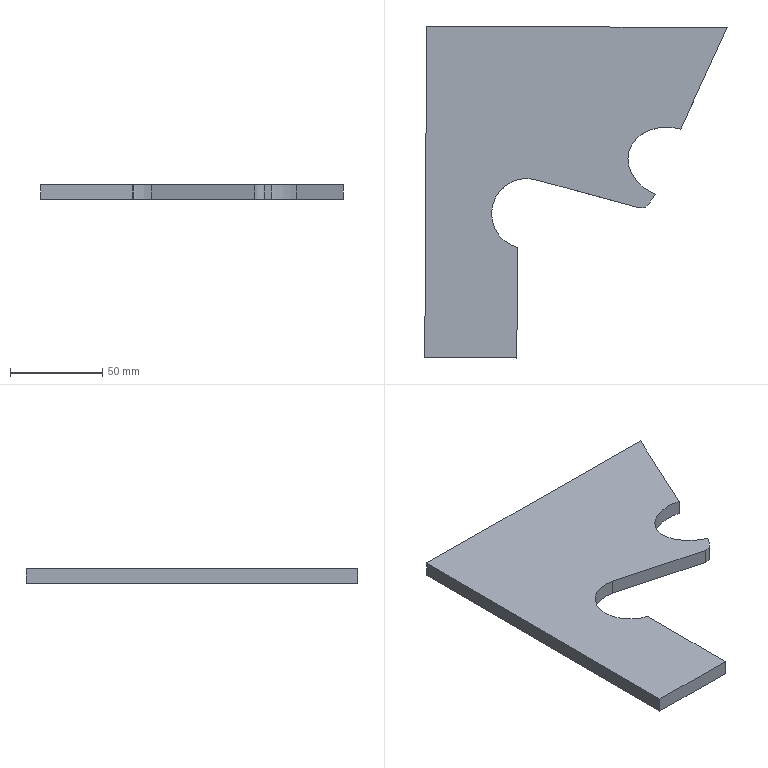Part | SolidWorks | features FlatPattern 1, SMBaseFlange 1, SheetMetal 1 | 1 solid | 14 faces | box 164.239 x 180.27 x 8 mm | volume 131142 mm3 | plane 9 | cylinder 3 | spline 2 | commonest cylinder face diameters 38.1 x2 10 x1
STEP:
#1=CARTESIAN_POINT('',(-214.283,4.192,8.));
#2=VERTEX_POINT('',#1);
#3=CARTESIAN_POINT('',(-190.247,22.578,8.));
#4=VERTEX_POINT('',#3);
#5=CARTESIAN_POINT('',(-195.233,4.192,8.));
#6=DIRECTION('',(0.,0.,-1.));
#7=DIRECTION('',(1.,0.,0.));
#8=AXIS2_PLACEMENT_3D('',#5,#6,#7);
#9=CIRCLE('',#8,19.05);
#10=EDGE_CURVE('',#2,#4,#9,.T.);
#11=ORIENTED_EDGE('',*,*,#10,.F.);
#12=CARTESIAN_POINT('',(-214.283,4.192,0.));
#13=VERTEX_POINT('',#12);
#14=CARTESIAN_POINT('',(-214.283,4.192,8.));
#15=DIRECTION('',(0.,0.,-1.));
#16=VECTOR('',#15,1000.);
#17=LINE('',#14,#16);
#18=EDGE_CURVE('',#2,#13,#17,.T.);
#19=ORIENTED_EDGE('',*,*,#18,.T.);
#20=CARTESIAN_POINT('',(-190.247,22.578,0.));
#21=VERTEX_POINT('',#20);
#22=CARTESIAN_POINT('',(-195.233,4.192,0.));
#23=DIRECTION('',(0.,0.,-1.));
#24=DIRECTION('',(1.,0.,0.));
#25=AXIS2_PLACEMENT_3D('',#22,#23,#24);
#26=CIRCLE('',#25,19.05);
#27=EDGE_CURVE('',#13,#21,#26,.T.);
#28=ORIENTED_EDGE('',*,*,#27,.T.);
#29=CARTESIAN_POINT('',(-190.247,22.578,8.));
#30=DIRECTION('',(0.,0.,-1.));
#31=VECTOR('',#30,1000.);
#32=LINE('',#29,#31);
#33=EDGE_CURVE('',#4,#21,#32,.T.);
#34=ORIENTED_EDGE('',*,*,#33,.F.);
#35=EDGE_LOOP('',(#11,#19,#28,#34));
#36=FACE_OUTER_BOUND('',#35,.T.);
#37=CARTESIAN_POINT('',(-195.233,4.192,8.));
#38=DIRECTION('',(0.,0.,-1.));
#39=DIRECTION('',(-1.,0.,0.));
#40=AXIS2_PLACEMENT_3D('',#37,#38,#39);
#41=CYLINDRICAL_SURFACE('',#40,19.05);
#42=ADVANCED_FACE('',(#36),#41,.F.);
#43=CARTESIAN_POINT('',(-139.675,37.946,8.));
#44=VERTEX_POINT('',#43);
#45=CARTESIAN_POINT('',(-111.658,50.087,8.));
#46=VERTEX_POINT('',#45);
#47=CARTESIAN_POINT('',(-139.675,37.946,8.));
#48=CARTESIAN_POINT('',(-136.754,48.717,8.));
#49=CARTESIAN_POINT('',(-125.15,53.746,8.));
#50=CARTESIAN_POINT('',(-111.658,50.087,8.));
#51=(BOUNDED_CURVE()B_SPLINE_CURVE(3,(#47,#48,#49,#50),.UNSPECIFIED.,.F.,.F.)B_SPLINE_CURVE_WITH_KNOTS((4,4),(0.,1.571),.UNSPECIFIED.)CURVE()GEOMETRIC_REPRESENTATION_ITEM()RATIONAL_B_SPLINE_CURVE((1.,0.8047,0.8047,1.))REPRESENTATION_ITEM(''));
#52=EDGE_CURVE('',#44,#46,#51,.T.);
#53=ORIENTED_EDGE('',*,*,#52,.F.);
#54=CARTESIAN_POINT('',(-139.675,37.946,0.));
#55=VERTEX_POINT('',#54);
#56=CARTESIAN_POINT('',(-139.675,37.946,8.));
#57=DIRECTION('',(0.,0.,-1.));
#58=VECTOR('',#57,1000.);
#59=LINE('',#56,#58);
#60=EDGE_CURVE('',#44,#55,#59,.T.);
#61=ORIENTED_EDGE('',*,*,#60,.T.);
#62=CARTESIAN_POINT('',(-111.658,50.087,0.));
#63=VERTEX_POINT('',#62);
#64=CARTESIAN_POINT('',(-139.675,37.946,0.));
#65=CARTESIAN_POINT('',(-136.754,48.717,0.));
#66=CARTESIAN_POINT('',(-125.15,53.746,0.));
#67=CARTESIAN_POINT('',(-111.658,50.087,0.));
#68=(BOUNDED_CURVE()B_SPLINE_CURVE(3,(#64,#65,#66,#67),.UNSPECIFIED.,.F.,.F.)B_SPLINE_CURVE_WITH_KNOTS((4,4),(0.,1.571),.UNSPECIFIED.)CURVE()GEOMETRIC_REPRESENTATION_ITEM()RATIONAL_B_SPLINE_CURVE((1.,0.8047,0.8047,1.))REPRESENTATION_ITEM(''));
#69=EDGE_CURVE('',#55,#63,#68,.T.);
#70=ORIENTED_EDGE('',*,*,#69,.T.);
#71=CARTESIAN_POINT('',(-111.658,50.087,8.));
#72=DIRECTION('',(0.,0.,-1.));
#73=VECTOR('',#72,1000.);
#74=LINE('',#71,#73);
#75=EDGE_CURVE('',#46,#63,#74,.T.);
#76=ORIENTED_EDGE('',*,*,#75,.F.);
#77=EDGE_LOOP('',(#53,#61,#70,#76));
#78=FACE_OUTER_BOUND('',#77,.T.);
#79=CARTESIAN_POINT('',(-139.675,37.946,8.));
#80=CARTESIAN_POINT('',(-139.675,37.946,0.));
#81=CARTESIAN_POINT('',(-136.754,48.717,8.));
#82=CARTESIAN_POINT('',(-136.754,48.717,0.));
#83=CARTESIAN_POINT('',(-125.15,53.746,8.));
#84=CARTESIAN_POINT('',(-125.15,53.746,0.));
#85=CARTESIAN_POINT('',(-111.658,50.087,8.));
#86=CARTESIAN_POINT('',(-111.658,50.087,0.));
#87=(BOUNDED_SURFACE()B_SPLINE_SURFACE(3,1,((#79,#80),(#81,#82),(#83,#84),(#85,#86)),.UNSPECIFIED.,.F.,.F.,.F.)B_SPLINE_SURFACE_WITH_KNOTS((4,4),(2,2),(0.,1.),(0.,1.),.UNSPECIFIED.)GEOMETRIC_REPRESENTATION_ITEM()RATIONAL_B_SPLINE_SURFACE(((1.,1.),(0.8047,0.8047),(0.8047,0.8047),(1.,1.)))REPRESENTATION_ITEM('')SURFACE());
#88=ADVANCED_FACE('',(#78),#87,.F.);
#89=ORIENTED_EDGE('',*,*,#60,.F.);
#90=CARTESIAN_POINT('',(-125.259,14.555,8.));
#91=VERTEX_POINT('',#90);
#92=CARTESIAN_POINT('',(-125.259,14.555,8.));
#93=CARTESIAN_POINT('',(-136.522,19.235,8.));
#94=CARTESIAN_POINT('',(-142.235,28.505,8.));
#95=CARTESIAN_POINT('',(-139.675,37.946,8.));
#96=(BOUNDED_CURVE()B_SPLINE_CURVE(3,(#92,#93,#94,#95),.UNSPECIFIED.,.F.,.F.)B_SPLINE_CURVE_WITH_KNOTS((4,4),(4.874,6.283),.UNSPECIFIED.)CURVE()GEOMETRIC_REPRESENTATION_ITEM()RATIONAL_B_SPLINE_CURVE((1.,0.8411,0.8411,1.))REPRESENTATION_ITEM(''));
#97=EDGE_CURVE('',#91,#44,#96,.T.);
#98=ORIENTED_EDGE('',*,*,#97,.F.);
#99=CARTESIAN_POINT('',(-125.259,14.555,0.));
#100=VERTEX_POINT('',#99);
#101=CARTESIAN_POINT('',(-125.259,14.555,8.));
#102=DIRECTION('',(0.,0.,-1.));
#103=VECTOR('',#102,1000.);
#104=LINE('',#101,#103);
#105=EDGE_CURVE('',#91,#100,#104,.T.);
#106=ORIENTED_EDGE('',*,*,#105,.T.);
#107=CARTESIAN_POINT('',(-125.259,14.555,0.));
#108=CARTESIAN_POINT('',(-136.522,19.235,0.));
#109=CARTESIAN_POINT('',(-142.235,28.505,0.));
#110=CARTESIAN_POINT('',(-139.675,37.946,0.));
#111=(BOUNDED_CURVE()B_SPLINE_CURVE(3,(#107,#108,#109,#110),.UNSPECIFIED.,.F.,.T.)B_SPLINE_CURVE_WITH_KNOTS((4,4),(4.874,6.283),.UNSPECIFIED.)CURVE()GEOMETRIC_REPRESENTATION_ITEM()RATIONAL_B_SPLINE_CURVE((1.,0.8411,0.8411,1.))REPRESENTATION_ITEM(''));
#112=EDGE_CURVE('',#100,#55,#111,.T.);
#113=ORIENTED_EDGE('',*,*,#112,.T.);
#114=EDGE_LOOP('',(#89,#98,#106,#113));
#115=FACE_OUTER_BOUND('',#114,.T.);
#116=CARTESIAN_POINT('',(-125.259,14.555,8.));
#117=CARTESIAN_POINT('',(-125.259,14.555,0.));
#118=CARTESIAN_POINT('',(-136.522,19.235,8.));
#119=CARTESIAN_POINT('',(-136.522,19.235,0.));
#120=CARTESIAN_POINT('',(-142.235,28.505,8.));
#121=CARTESIAN_POINT('',(-142.235,28.505,0.));
#122=CARTESIAN_POINT('',(-139.675,37.946,8.));
#123=CARTESIAN_POINT('',(-139.675,37.946,0.));
#124=(BOUNDED_SURFACE()B_SPLINE_SURFACE(3,1,((#116,#117),(#118,#119),(#120,#121),(#122,#123)),.UNSPECIFIED.,.F.,.F.,.F.)B_SPLINE_SURFACE_WITH_KNOTS((4,4),(2,2),(0.,1.),(0.,1.),.UNSPECIFIED.)GEOMETRIC_REPRESENTATION_ITEM()RATIONAL_B_SPLINE_SURFACE(((1.,1.),(0.8411,0.8411),(0.8411,0.8411),(1.,1.)))REPRESENTATION_ITEM('')SURFACE());
#125=ADVANCED_FACE('',(#115),#124,.F.);
#126=CARTESIAN_POINT('',(-86.305,105.187,0.));
#127=VERTEX_POINT('',#126);
#128=CARTESIAN_POINT('',(-86.305,105.187,0.));
#129=DIRECTION('',(0.418,0.9084,0.));
#130=VECTOR('',#129,1000.);
#131=LINE('',#128,#130);
#132=EDGE_CURVE('',#63,#127,#131,.T.);
#133=ORIENTED_EDGE('',*,*,#132,.T.);
#134=CARTESIAN_POINT('',(-86.305,105.187,8.));
#135=VERTEX_POINT('',#134);
#136=CARTESIAN_POINT('',(-86.305,105.187,8.));
#137=DIRECTION('',(0.,0.,-1.));
#138=VECTOR('',#137,1000.);
#139=LINE('',#136,#138);
#140=EDGE_CURVE('',#135,#127,#139,.T.);
#141=ORIENTED_EDGE('',*,*,#140,.F.);
#142=CARTESIAN_POINT('',(-86.305,105.187,8.));
#143=DIRECTION('',(0.418,0.9084,0.));
#144=VECTOR('',#143,1000.);
#145=LINE('',#142,#144);
#146=EDGE_CURVE('',#46,#135,#145,.T.);
#147=ORIENTED_EDGE('',*,*,#146,.F.);
#148=ORIENTED_EDGE('',*,*,#75,.T.);
#149=EDGE_LOOP('',(#133,#141,#147,#148));
#150=FACE_OUTER_BOUND('',#149,.T.);
#151=CARTESIAN_POINT('',(-86.305,105.187,8.));
#152=DIRECTION('',(-0.9084,0.418,0.));
#153=DIRECTION('',(-0.418,-0.9084,0.));
#154=AXIS2_PLACEMENT_3D('',#151,#152,#153);
#155=PLANE('',#154);
#156=ADVANCED_FACE('',(#150),#155,.F.);
#157=CARTESIAN_POINT('',(-249.564,106.077,0.));
#158=VERTEX_POINT('',#157);
#159=CARTESIAN_POINT('',(-249.564,106.077,0.));
#160=DIRECTION('',(-1.,0.005451,0.));
#161=VECTOR('',#160,1000.);
#162=LINE('',#159,#161);
#163=EDGE_CURVE('',#127,#158,#162,.T.);
#164=ORIENTED_EDGE('',*,*,#163,.T.);
#165=CARTESIAN_POINT('',(-249.564,106.077,8.));
#166=VERTEX_POINT('',#165);
#167=CARTESIAN_POINT('',(-249.564,106.077,8.));
#168=DIRECTION('',(0.,0.,-1.));
#169=VECTOR('',#168,1000.);
#170=LINE('',#167,#169);
#171=EDGE_CURVE('',#166,#158,#170,.T.);
#172=ORIENTED_EDGE('',*,*,#171,.F.);
#173=CARTESIAN_POINT('',(-249.564,106.077,8.));
#174=DIRECTION('',(-1.,0.005451,0.));
#175=VECTOR('',#174,1000.);
#176=LINE('',#173,#175);
#177=EDGE_CURVE('',#135,#166,#176,.T.);
#178=ORIENTED_EDGE('',*,*,#177,.F.);
#179=ORIENTED_EDGE('',*,*,#140,.T.);
#180=EDGE_LOOP('',(#164,#172,#178,#179));
#181=FACE_OUTER_BOUND('',#180,.T.);
#182=CARTESIAN_POINT('',(-249.564,106.077,8.));
#183=DIRECTION('',(-0.005451,-1.,0.));
#184=DIRECTION('',(1.,-0.005451,0.));
#185=AXIS2_PLACEMENT_3D('',#182,#183,#184);
#186=PLANE('',#185);
#187=ADVANCED_FACE('',(#181),#186,.F.);
#188=CARTESIAN_POINT('',(-250.545,-73.921,0.));
#189=VERTEX_POINT('',#188);
#190=CARTESIAN_POINT('',(-250.545,-73.921,0.));
#191=DIRECTION('',(-0.005451,-1.,0.));
#192=VECTOR('',#191,1000.);
#193=LINE('',#190,#192);
#194=EDGE_CURVE('',#158,#189,#193,.T.);
#195=ORIENTED_EDGE('',*,*,#194,.T.);
#196=CARTESIAN_POINT('',(-250.545,-73.921,8.));
#197=VERTEX_POINT('',#196);
#198=CARTESIAN_POINT('',(-250.545,-73.921,8.));
#199=DIRECTION('',(0.,0.,-1.));
#200=VECTOR('',#199,1000.);
#201=LINE('',#198,#200);
#202=EDGE_CURVE('',#197,#189,#201,.T.);
#203=ORIENTED_EDGE('',*,*,#202,.F.);
#204=CARTESIAN_POINT('',(-250.545,-73.921,8.));
#205=DIRECTION('',(-0.005451,-1.,0.));
#206=VECTOR('',#205,1000.);
#207=LINE('',#204,#206);
#208=EDGE_CURVE('',#166,#197,#207,.T.);
#209=ORIENTED_EDGE('',*,*,#208,.F.);
#210=ORIENTED_EDGE('',*,*,#171,.T.);
#211=EDGE_LOOP('',(#195,#203,#209,#210));
#212=FACE_OUTER_BOUND('',#211,.T.);
#213=CARTESIAN_POINT('',(-250.545,-73.921,8.));
#214=DIRECTION('',(1.,-0.005451,0.));
#215=DIRECTION('',(0.005451,1.,0.));
#216=AXIS2_PLACEMENT_3D('',#213,#214,#215);
#217=PLANE('',#216);
#218=ADVANCED_FACE('',(#212),#217,.F.);
#219=CARTESIAN_POINT('',(-200.545,-74.193,0.));
#220=VERTEX_POINT('',#219);
#221=CARTESIAN_POINT('',(-200.545,-74.193,0.));
#222=DIRECTION('',(1.,-0.005451,0.));
#223=VECTOR('',#222,1000.);
#224=LINE('',#221,#223);
#225=EDGE_CURVE('',#189,#220,#224,.T.);
#226=ORIENTED_EDGE('',*,*,#225,.T.);
#227=CARTESIAN_POINT('',(-200.545,-74.193,8.));
#228=VERTEX_POINT('',#227);
#229=CARTESIAN_POINT('',(-200.545,-74.193,8.));
#230=DIRECTION('',(0.,0.,-1.));
#231=VECTOR('',#230,1000.);
#232=LINE('',#229,#231);
#233=EDGE_CURVE('',#228,#220,#232,.T.);
#234=ORIENTED_EDGE('',*,*,#233,.F.);
#235=CARTESIAN_POINT('',(-200.545,-74.193,8.));
#236=DIRECTION('',(1.,-0.005451,0.));
#237=VECTOR('',#236,1000.);
#238=LINE('',#235,#237);
#239=EDGE_CURVE('',#197,#228,#238,.T.);
#240=ORIENTED_EDGE('',*,*,#239,.F.);
#241=ORIENTED_EDGE('',*,*,#202,.T.);
#242=EDGE_LOOP('',(#226,#234,#240,#241));
#243=FACE_OUTER_BOUND('',#242,.T.);
#244=CARTESIAN_POINT('',(-200.545,-74.193,8.));
#245=DIRECTION('',(0.005451,1.,0.));
#246=DIRECTION('',(-1.,0.005451,0.));
#247=AXIS2_PLACEMENT_3D('',#244,#245,#246);
#248=PLANE('',#247);
#249=ADVANCED_FACE('',(#243),#248,.F.);
#250=CARTESIAN_POINT('',(-200.218,-14.194,0.));
#251=VERTEX_POINT('',#250);
#252=CARTESIAN_POINT('',(-200.218,-14.194,0.));
#253=DIRECTION('',(0.005451,1.,0.));
#254=VECTOR('',#253,1000.);
#255=LINE('',#252,#254);
#256=EDGE_CURVE('',#220,#251,#255,.T.);
#257=ORIENTED_EDGE('',*,*,#256,.T.);
#258=CARTESIAN_POINT('',(-200.218,-14.194,8.));
#259=VERTEX_POINT('',#258);
#260=CARTESIAN_POINT('',(-200.218,-14.194,8.));
#261=DIRECTION('',(0.,0.,-1.));
#262=VECTOR('',#261,1000.);
#263=LINE('',#260,#262);
#264=EDGE_CURVE('',#259,#251,#263,.T.);
#265=ORIENTED_EDGE('',*,*,#264,.F.);
#266=CARTESIAN_POINT('',(-200.218,-14.194,8.));
#267=DIRECTION('',(0.005451,1.,0.));
#268=VECTOR('',#267,1000.);
#269=LINE('',#266,#268);
#270=EDGE_CURVE('',#228,#259,#269,.T.);
#271=ORIENTED_EDGE('',*,*,#270,.F.);
#272=ORIENTED_EDGE('',*,*,#233,.T.);
#273=EDGE_LOOP('',(#257,#265,#271,#272));
#274=FACE_OUTER_BOUND('',#273,.T.);
#275=CARTESIAN_POINT('',(-200.218,-14.194,8.));
#276=DIRECTION('',(-1.,0.005451,0.));
#277=DIRECTION('',(-0.005451,-1.,0.));
#278=AXIS2_PLACEMENT_3D('',#275,#276,#277);
#279=PLANE('',#278);
#280=ADVANCED_FACE('',(#274),#279,.F.);
#281=ORIENTED_EDGE('',*,*,#18,.F.);
#282=CARTESIAN_POINT('',(-195.233,4.192,8.));
#283=DIRECTION('',(0.,0.,-1.));
#284=DIRECTION('',(1.,0.,0.));
#285=AXIS2_PLACEMENT_3D('',#282,#283,#284);
#286=CIRCLE('',#285,19.05);
#287=EDGE_CURVE('',#259,#2,#286,.T.);
#288=ORIENTED_EDGE('',*,*,#287,.F.);
#289=ORIENTED_EDGE('',*,*,#264,.T.);
#290=CARTESIAN_POINT('',(-195.233,4.192,0.));
#291=DIRECTION('',(0.,0.,-1.));
#292=DIRECTION('',(1.,0.,0.));
#293=AXIS2_PLACEMENT_3D('',#290,#291,#292);
#294=CIRCLE('',#293,19.05);
#295=EDGE_CURVE('',#251,#13,#294,.T.);
#296=ORIENTED_EDGE('',*,*,#295,.T.);
#297=EDGE_LOOP('',(#281,#288,#289,#296));
#298=FACE_OUTER_BOUND('',#297,.T.);
#299=CARTESIAN_POINT('',(-195.233,4.192,8.));
#300=DIRECTION('',(0.,0.,-1.));
#301=DIRECTION('',(-1.,0.,0.));
#302=AXIS2_PLACEMENT_3D('',#299,#300,#301);
#303=CYLINDRICAL_SURFACE('',#302,19.05);
#304=ADVANCED_FACE('',(#298),#303,.F.);
#305=CARTESIAN_POINT('',(-134.403,7.436,0.));
#306=VERTEX_POINT('',#305);
#307=CARTESIAN_POINT('',(-134.403,7.436,0.));
#308=DIRECTION('',(0.9651,-0.2617,0.));
#309=VECTOR('',#308,1000.);
#310=LINE('',#307,#309);
#311=EDGE_CURVE('',#21,#306,#310,.T.);
#312=ORIENTED_EDGE('',*,*,#311,.T.);
#313=CARTESIAN_POINT('',(-134.403,7.436,8.));
#314=VERTEX_POINT('',#313);
#315=CARTESIAN_POINT('',(-134.403,7.436,8.));
#316=DIRECTION('',(0.,0.,-1.));
#317=VECTOR('',#316,1000.);
#318=LINE('',#315,#317);
#319=EDGE_CURVE('',#314,#306,#318,.T.);
#320=ORIENTED_EDGE('',*,*,#319,.F.);
#321=CARTESIAN_POINT('',(-134.403,7.436,8.));
#322=DIRECTION('',(0.9651,-0.2617,0.));
#323=VECTOR('',#322,1000.);
#324=LINE('',#321,#323);
#325=EDGE_CURVE('',#4,#314,#324,.T.);
#326=ORIENTED_EDGE('',*,*,#325,.F.);
#327=ORIENTED_EDGE('',*,*,#33,.T.);
#328=EDGE_LOOP('',(#312,#320,#326,#327));
#329=FACE_OUTER_BOUND('',#328,.T.);
#330=CARTESIAN_POINT('',(-134.403,7.436,8.));
#331=DIRECTION('',(0.2617,0.9651,0.));
#332=DIRECTION('',(-0.9651,0.2617,0.));
#333=AXIS2_PLACEMENT_3D('',#330,#331,#332);
#334=PLANE('',#333);
#335=ADVANCED_FACE('',(#329),#334,.F.);
#336=CARTESIAN_POINT('',(-129.045,9.328,0.));
#337=VERTEX_POINT('',#336);
#338=CARTESIAN_POINT('',(-133.094,12.261,0.));
#339=DIRECTION('',(0.,0.,1.));
#340=DIRECTION('',(-1.,0.,0.));
#341=AXIS2_PLACEMENT_3D('',#338,#339,#340);
#342=CIRCLE('',#341,5.);
#343=EDGE_CURVE('',#306,#337,#342,.T.);
#344=ORIENTED_EDGE('',*,*,#343,.T.);
#345=CARTESIAN_POINT('',(-129.045,9.328,8.));
#346=VERTEX_POINT('',#345);
#347=CARTESIAN_POINT('',(-129.045,9.328,8.));
#348=DIRECTION('',(0.,0.,-1.));
#349=VECTOR('',#348,1000.);
#350=LINE('',#347,#349);
#351=EDGE_CURVE('',#346,#337,#350,.T.);
#352=ORIENTED_EDGE('',*,*,#351,.F.);
#353=CARTESIAN_POINT('',(-133.094,12.261,8.));
#354=DIRECTION('',(0.,0.,1.));
#355=DIRECTION('',(-1.,0.,0.));
#356=AXIS2_PLACEMENT_3D('',#353,#354,#355);
#357=CIRCLE('',#356,5.);
#358=EDGE_CURVE('',#314,#346,#357,.T.);
#359=ORIENTED_EDGE('',*,*,#358,.F.);
#360=ORIENTED_EDGE('',*,*,#319,.T.);
#361=EDGE_LOOP('',(#344,#352,#359,#360));
#362=FACE_OUTER_BOUND('',#361,.T.);
#363=CARTESIAN_POINT('',(-133.094,12.261,8.));
#364=DIRECTION('',(0.,0.,-1.));
#365=DIRECTION('',(-1.,0.,0.));
#366=AXIS2_PLACEMENT_3D('',#363,#364,#365);
#367=CYLINDRICAL_SURFACE('',#366,5.);
#368=ADVANCED_FACE('',(#362),#367,.T.);
#369=CARTESIAN_POINT('',(-129.045,9.328,0.));
#370=DIRECTION('',(0.5866,0.8099,0.));
#371=VECTOR('',#370,1000.);
#372=LINE('',#369,#371);
#373=EDGE_CURVE('',#337,#100,#372,.T.);
#374=ORIENTED_EDGE('',*,*,#373,.T.);
#375=ORIENTED_EDGE('',*,*,#105,.F.);
#376=CARTESIAN_POINT('',(-129.045,9.328,8.));
#377=DIRECTION('',(0.5866,0.8099,0.));
#378=VECTOR('',#377,1000.);
#379=LINE('',#376,#378);
#380=EDGE_CURVE('',#346,#91,#379,.T.);
#381=ORIENTED_EDGE('',*,*,#380,.F.);
#382=ORIENTED_EDGE('',*,*,#351,.T.);
#383=EDGE_LOOP('',(#374,#375,#381,#382));
#384=FACE_OUTER_BOUND('',#383,.T.);
#385=CARTESIAN_POINT('',(-129.045,9.328,8.));
#386=DIRECTION('',(-0.8099,0.5866,0.));
#387=DIRECTION('',(-0.5866,-0.8099,0.));
#388=AXIS2_PLACEMENT_3D('',#385,#386,#387);
#389=PLANE('',#388);
#390=ADVANCED_FACE('',(#384),#389,.F.);
#391=ORIENTED_EDGE('',*,*,#97,.T.);
#392=ORIENTED_EDGE('',*,*,#52,.T.);
#393=ORIENTED_EDGE('',*,*,#146,.T.);
#394=ORIENTED_EDGE('',*,*,#177,.T.);
#395=ORIENTED_EDGE('',*,*,#208,.T.);
#396=ORIENTED_EDGE('',*,*,#239,.T.);
#397=ORIENTED_EDGE('',*,*,#270,.T.);
#398=ORIENTED_EDGE('',*,*,#287,.T.);
#399=ORIENTED_EDGE('',*,*,#10,.T.);
#400=ORIENTED_EDGE('',*,*,#325,.T.);
#401=ORIENTED_EDGE('',*,*,#358,.T.);
#402=ORIENTED_EDGE('',*,*,#380,.T.);
#403=EDGE_LOOP('',(#391,#392,#393,#394,#395,#396,#397,#398,#399,#400,#401,#402));
#404=FACE_OUTER_BOUND('',#403,.T.);
#405=CARTESIAN_POINT('',(-116.644,31.701,8.));
#406=DIRECTION('',(0.,0.,1.));
#407=DIRECTION('',(1.,0.,0.));
#408=AXIS2_PLACEMENT_3D('',#405,#406,#407);
#409=PLANE('',#408);
#410=ADVANCED_FACE('',(#404),#409,.T.);
#411=ORIENTED_EDGE('',*,*,#112,.F.);
#412=ORIENTED_EDGE('',*,*,#373,.F.);
#413=ORIENTED_EDGE('',*,*,#343,.F.);
#414=ORIENTED_EDGE('',*,*,#311,.F.);
#415=ORIENTED_EDGE('',*,*,#27,.F.);
#416=ORIENTED_EDGE('',*,*,#295,.F.);
#417=ORIENTED_EDGE('',*,*,#256,.F.);
#418=ORIENTED_EDGE('',*,*,#225,.F.);
#419=ORIENTED_EDGE('',*,*,#194,.F.);
#420=ORIENTED_EDGE('',*,*,#163,.F.);
#421=ORIENTED_EDGE('',*,*,#132,.F.);
#422=ORIENTED_EDGE('',*,*,#69,.F.);
#423=EDGE_LOOP('',(#411,#412,#413,#414,#415,#416,#417,#418,#419,#420,#421,#422));
#424=FACE_OUTER_BOUND('',#423,.T.);
#425=CARTESIAN_POINT('',(-116.644,31.701,0.));
#426=DIRECTION('',(0.,0.,1.));
#427=DIRECTION('',(1.,0.,0.));
#428=AXIS2_PLACEMENT_3D('',#425,#426,#427);
#429=PLANE('',#428);
#430=ADVANCED_FACE('',(#424),#429,.F.);
#431=CLOSED_SHELL('',(#42,#88,#125,#156,#187,#218,#249,#280,#304,#335,#368,#390,#410,#430));
#432=MANIFOLD_SOLID_BREP('',#431);
#433=CARTESIAN_POINT('',(0.,0.,0.));
#434=DIRECTION('',(0.,0.,1.));
#435=DIRECTION('',(1.,0.,0.));
#436=AXIS2_PLACEMENT_3D('',#433,#434,#435);
#437=(LENGTH_UNIT()NAMED_UNIT(*)SI_UNIT(.MILLI.,.METRE.));
#438=UNCERTAINTY_MEASURE_WITH_UNIT(LENGTH_MEASURE(0.00001),#437,'','');
#439=(NAMED_UNIT(*)PLANE_ANGLE_UNIT()SI_UNIT($,.RADIAN.));
#440=(NAMED_UNIT(*)SI_UNIT($,.STERADIAN.)SOLID_ANGLE_UNIT());
#441=(GEOMETRIC_REPRESENTATION_CONTEXT(3)GLOBAL_UNCERTAINTY_ASSIGNED_CONTEXT((#438))GLOBAL_UNIT_ASSIGNED_CONTEXT((#437,#439,#440))REPRESENTATION_CONTEXT('',''));
#442=ADVANCED_BREP_SHAPE_REPRESENTATION('',(#432,#436),#441);